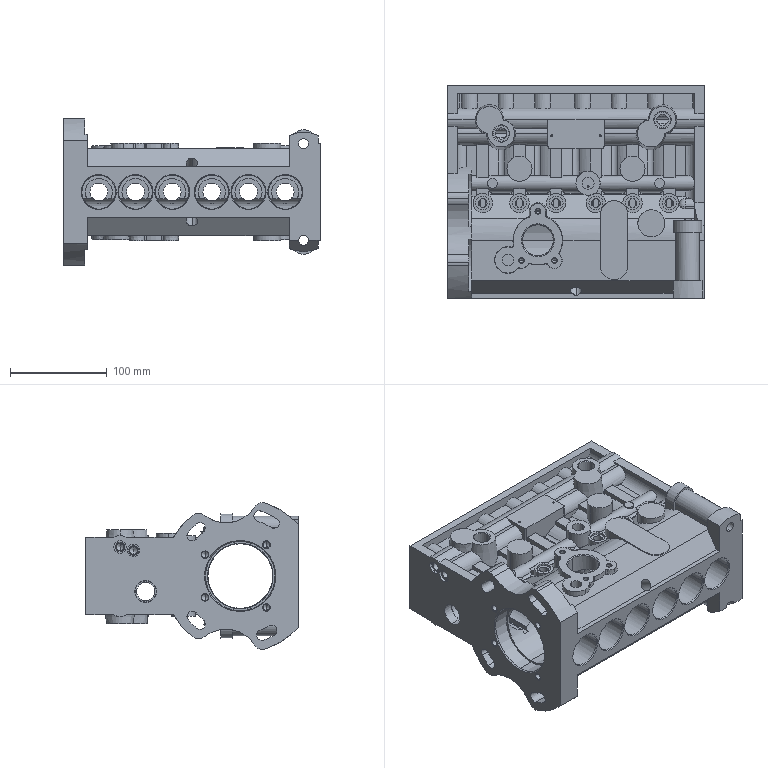Part | SolidWorks | features BaseBody 1 | 1 solid | 1098 faces | box 266 x 220 x 152.149 mm | volume 2634988 mm3 | cylinder 531 | plane 303 | cone 258 | sphere 4 | torus 2 | commonest cylinder face diameters 20 x46 52 x40 35 x30 28 x27 12.5 x26 10.2 x24